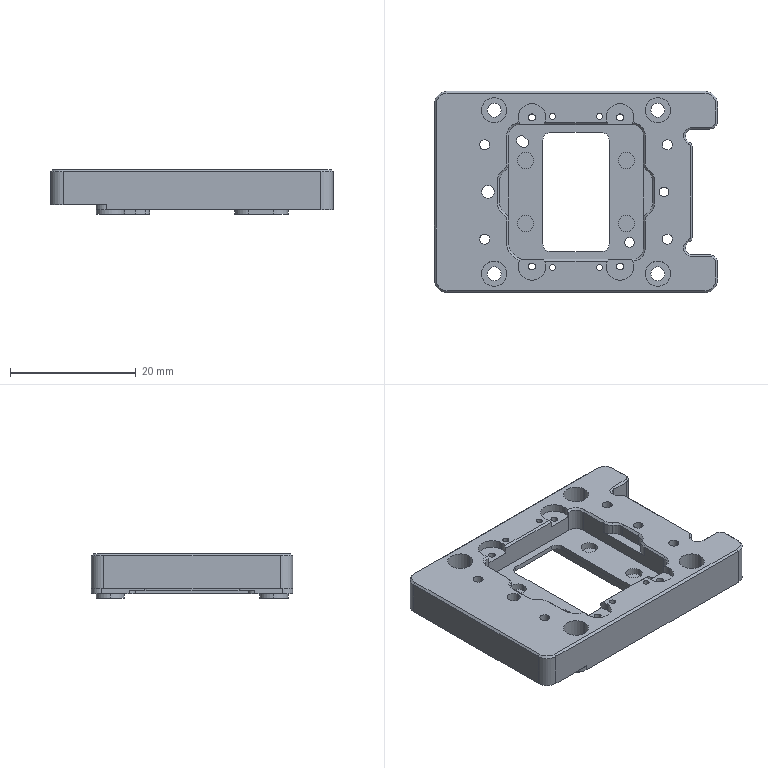NC program | NX | posted with a generic post | part box 45 x 32 x 7.05 mm
Lines 3844 to 5415 of 5787, first 1338 of 1564 lines:
(HOLE_MILLING_COPY , TOOL : D1.5)
N7602 T19 M6
N7604 G54
N7606 G17 G0 G90 X-8. Y5. S9500 M3
N7608 G43 Z30. H19
N7610 Z-3.35
N7612 G94 G3 X-7.725 Y4.725 R0.275 F950.
N7614 X-7.45 Y5. R0.275
N7616 X-7.45 Y5. Z-3.45 I-0.55 J0.
N7618 X-7.45 Y5. Z-3.55 I-0.55 J0.
N7620 X-7.45 Y5. Z-3.65 I-0.55 J0.
N7622 X-7.45 Y5. Z-3.75 I-0.55 J0.
N7624 X-7.45 Y5. Z-3.85 I-0.55 J0.
N7626 X-7.45 Y5. Z-3.95 I-0.55 J0.
N7628 X-7.45 Y5. Z-4.05 I-0.55 J0.
N7630 X-7.45 Y5. Z-4.15 I-0.55 J0.
N7632 X-7.45 Y5. Z-4.25 I-0.55 J0.
N7634 X-7.45 Y5. Z-4.35 I-0.55 J0.
N7636 X-7.45 Y5. Z-4.45 I-0.55 J0.
N7638 X-7.45 Y5. Z-4.55 I-0.55 J0.
N7640 X-7.45 Y5. Z-4.65 I-0.55 J0.
N7642 X-7.45 Y5. Z-4.75 I-0.55 J0.
N7644 X-7.45 Y5. Z-4.85 I-0.55 J0.
N7646 X-8.55 Y5. Z-4.9 I-0.55 J0.
N7648 X-8. Y4.45 R0.55
N7650 X-8.55 Y5. R-0.55
N7652 X-8.275 Y4.725 R0.275
N7654 X-8. Y5. R0.275
N7656 G0 Z30.
N7658 Y-5.
N7660 Z-3.35
N7662 G3 X-7.725 Y-5.275 R0.275
N7664 X-7.45 Y-5. R0.275
N7666 X-7.45 Y-5. Z-3.45 I-0.55 J0.
N7668 X-7.45 Y-5. Z-3.55 I-0.55 J0.
N7670 X-7.45 Y-5. Z-3.65 I-0.55 J0.
N7672 X-7.45 Y-5. Z-3.75 I-0.55 J0.
N7674 X-7.45 Y-5. Z-3.85 I-0.55 J0.
N7676 X-7.45 Y-5. Z-3.95 I-0.55 J0.
N7678 X-7.45 Y-5. Z-4.05 I-0.55 J0.
N7680 X-7.45 Y-5. Z-4.15 I-0.55 J0.
N7682 X-7.45 Y-5. Z-4.25 I-0.55 J0.
N7684 X-7.45 Y-5. Z-4.35 I-0.55 J0.
N7686 X-7.45 Y-5. Z-4.45 I-0.55 J0.
N7688 X-7.45 Y-5. Z-4.55 I-0.55 J0.
N7690 X-7.45 Y-5. Z-4.65 I-0.55 J0.
N7692 X-7.45 Y-5. Z-4.75 I-0.55 J0.
N7694 X-7.45 Y-5. Z-4.85 I-0.55 J0.
N7696 X-8.55 Y-5. Z-4.9 I-0.55 J0.
N7698 X-8. Y-5.55 R0.55
N7700 X-8.55 Y-5. R-0.55
N7702 X-8.275 Y-5.275 R0.275
N7704 X-8. Y-5. R0.275
N7706 G0 Z30.
N7708 X8.
N7710 Z-3.35
N7712 G3 X8.275 Y-5.275 R0.275
N7714 X8.55 Y-5. R0.275
N7716 X8.55 Y-5. Z-3.45 I-0.55 J0.
N7718 X8.55 Y-5. Z-3.55 I-0.55 J0.
N7720 X8.55 Y-5. Z-3.65 I-0.55 J0.
N7722 X8.55 Y-5. Z-3.75 I-0.55 J0.
N7724 X8.55 Y-5. Z-3.85 I-0.55 J0.
N7726 X8.55 Y-5. Z-3.95 I-0.55 J0.
N7728 X8.55 Y-5. Z-4.05 I-0.55 J0.
N7730 X8.55 Y-5. Z-4.15 I-0.55 J0.
N7732 X8.55 Y-5. Z-4.25 I-0.55 J0.
N7734 X8.55 Y-5. Z-4.35 I-0.55 J0.
N7736 X8.55 Y-5. Z-4.45 I-0.55 J0.
N7738 X8.55 Y-5. Z-4.55 I-0.55 J0.
N7740 X8.55 Y-5. Z-4.65 I-0.55 J0.
N7742 X8.55 Y-5. Z-4.75 I-0.55 J0.
N7744 X8.55 Y-5. Z-4.85 I-0.55 J0.
N7746 X7.45 Y-5. Z-4.9 I-0.55 J0.
N7748 X8. Y-5.55 R0.55
N7750 X7.45 Y-5. R-0.55
N7752 X7.725 Y-5.275 R0.275
N7754 X8. Y-5. R0.275
N7756 G0 Z30.
N7758 Y5.
N7760 Z-3.35
N7762 G3 X8.275 Y4.725 R0.275
N7764 X8.55 Y5. R0.275
N7766 X8.55 Y5. Z-3.45 I-0.55 J0.
N7768 X8.55 Y5. Z-3.55 I-0.55 J0.
N7770 X8.55 Y5. Z-3.65 I-0.55 J0.
N7772 X8.55 Y5. Z-3.75 I-0.55 J0.
N7774 X8.55 Y5. Z-3.85 I-0.55 J0.
N7776 X8.55 Y5. Z-3.95 I-0.55 J0.
N7778 X8.55 Y5. Z-4.05 I-0.55 J0.
N7780 X8.55 Y5. Z-4.15 I-0.55 J0.
N7782 X8.55 Y5. Z-4.25 I-0.55 J0.
N7784 X8.55 Y5. Z-4.35 I-0.55 J0.
N7786 X8.55 Y5. Z-4.45 I-0.55 J0.
N7788 X8.55 Y5. Z-4.55 I-0.55 J0.
N7790 X8.55 Y5. Z-4.65 I-0.55 J0.
N7792 X8.55 Y5. Z-4.75 I-0.55 J0.
N7794 X8.55 Y5. Z-4.85 I-0.55 J0.
N7796 X7.45 Y5. Z-4.9 I-0.55 J0.
N7798 X8. Y4.45 R0.55
N7800 X7.45 Y5. R-0.55
N7802 X7.725 Y4.725 R0.275
N7804 X8. Y5. R0.275
N7806 G0 Z30.
(CAVITY_MILL_COPY , TOOL : D1.5)
N7808 X-4.2 Y-7.103
N7810 Z-4.
N7812 G3 X-4.5 Y-7.817 R1.
N7814 G1 Y-8.25
N7816 G3 X-4. Y-8.75 R0.5
N7818 G1 X-3.567
N7820 G3 X-2.853 Y-8.45 R1.
N7822 G0 X-4.2 Y-7.103 Z-4.15
N7824 G3 X-4.5 Y-7.817 R1.
N7826 G1 Y-8.25
N7828 G3 X-4. Y-8.75 R0.5
N7830 G1 X-3.567
N7832 G3 X-2.853 Y-8.45 R1.
N7834 G0 X-4.2 Y-7.103 Z-4.3
N7836 G3 X-4.5 Y-7.817 R1.
N7838 G1 Y-8.25
N7840 G3 X-4. Y-8.75 R0.5
N7842 G1 X-3.567
N7844 G3 X-2.853 Y-8.45 R1.
N7846 G0 X-4.2 Y-7.103 Z-4.45
N7848 G3 X-4.5 Y-7.817 R1.
N7850 G1 Y-8.25
N7852 G3 X-4. Y-8.75 R0.5
N7854 G1 X-3.567
N7856 G3 X-2.853 Y-8.45 R1.
N7858 G0 X-4.2 Y-7.104 Z-4.6
N7860 G3 X-4.5 Y-7.818 R1.
N7862 G1 Y-8.25
N7864 G3 X-4. Y-8.75 R0.5
N7866 G1 X-3.568
N7868 G3 X-2.854 Y-8.45 R1.
N7870 G0 Z30.
N7872 X2.853
N7874 Z-4.
N7876 G3 X3.567 Y-8.75 R1.
N7878 G1 X4.
N7880 G3 X4.5 Y-8.25 R0.5
N7882 G1 Y-7.817
N7884 G3 X4.2 Y-7.103 R1.
N7886 G0 X2.853 Y-8.45 Z-4.15
N7888 G3 X3.567 Y-8.75 R1.
N7890 G1 X4.
N7892 G3 X4.5 Y-8.25 R0.5
N7894 G1 Y-7.817
N7896 G3 X4.2 Y-7.103 R1.
N7898 G0 X2.853 Y-8.45 Z-4.3
N7900 G3 X3.567 Y-8.75 R1.
N7902 G1 X4.
N7904 G3 X4.5 Y-8.25 R0.5
N7906 G1 Y-7.817
N7908 G3 X4.2 Y-7.103 R1.
N7910 G0 X2.853 Y-8.45 Z-4.45
N7912 G3 X3.567 Y-8.75 R1.
N7914 G1 X4.
N7916 G3 X4.5 Y-8.25 R0.5
N7918 G1 Y-7.817
N7920 G3 X4.2 Y-7.103 R1.
N7922 G0 X2.854 Y-8.45 Z-4.6
N7924 G3 X3.568 Y-8.75 R1.
N7926 G1 X4.
N7928 G3 X4.5 Y-8.25 R0.5
N7930 G1 Y-7.818
N7932 G3 X4.2 Y-7.104 R1.
N7934 G0 Z30.
N7936 Y7.103
N7938 Z-4.
N7940 G3 X4.5 Y7.817 R1.
N7942 G1 Y8.25
N7944 G3 X4. Y8.75 R0.5
N7946 G1 X3.567
N7948 G3 X2.853 Y8.45 R1.
N7950 G0 X4.2 Y7.103 Z-4.15
N7952 G3 X4.5 Y7.817 R1.
N7954 G1 Y8.25
N7956 G3 X4. Y8.75 R0.5
N7958 G1 X3.567
N7960 G3 X2.853 Y8.45 R1.
N7962 G0 X4.2 Y7.103 Z-4.3
N7964 G3 X4.5 Y7.817 R1.
N7966 G1 Y8.25
N7968 G3 X4. Y8.75 R0.5
N7970 G1 X3.567
N7972 G3 X2.853 Y8.45 R1.
N7974 G0 X4.2 Y7.103 Z-4.45
N7976 G3 X4.5 Y7.817 R1.
N7978 G1 Y8.25
N7980 G3 X4. Y8.75 R0.5
N7982 G1 X3.567
N7984 G3 X2.853 Y8.45 R1.
N7986 G0 X4.2 Y7.103 Z-4.6
N7988 G3 X4.5 Y7.817 R1.
N7990 G1 Y8.25
N7992 G3 X4. Y8.75 R0.5
N7994 G1 X3.567
N7996 G3 X2.853 Y8.45 R1.
N7998 G0 Z30.
N8000 X-2.853
N8002 Z-4.
N8004 G3 X-3.567 Y8.75 R1.
N8006 G1 X-4.
N8008 G3 X-4.5 Y8.25 R0.5
N8010 G1 Y7.817
N8012 G3 X-4.2 Y7.103 R1.
N8014 G0 X-2.853 Y8.45 Z-4.15
N8016 G3 X-3.567 Y8.75 R1.
N8018 G1 X-4.
N8020 G3 X-4.5 Y8.25 R0.5
N8022 G1 Y7.817
N8024 G3 X-4.2 Y7.103 R1.
N8026 G0 X-2.853 Y8.45 Z-4.3
N8028 G3 X-3.567 Y8.75 R1.
N8030 G1 X-4.
N8032 G3 X-4.5 Y8.25 R0.5
N8034 G1 Y7.817
N8036 G3 X-4.2 Y7.103 R1.
N8038 G0 X-2.853 Y8.45 Z-4.45
N8040 G3 X-3.567 Y8.75 R1.
N8042 G1 X-4.
N8044 G3 X-4.5 Y8.25 R0.5
N8046 G1 Y7.817
N8048 G3 X-4.2 Y7.103 R1.
N8050 G0 X-2.853 Y8.45 Z-4.6
N8052 G3 X-3.567 Y8.75 R1.
N8054 G1 X-4.
N8056 G3 X-4.5 Y8.25 R0.5
N8058 G1 Y7.817
N8060 G3 X-4.2 Y7.103 R1.
N8062 G0 Z30.
(CAVITY_MILL_COPY_COPY , TOOL : D1.5)
N8064 X20.107 Y9.111
N8066 Z-0.139
N8068 G3 X19.393 Y9.411 R1.
N8070 G1 X18.5
N8072 G3 X18.257 Y8.451 R0.511
N8074 G2 X18.811 Y7.952 R1.589
N8076 G3 X19.317 Y7.569 R1.
N8078 G0 X20.404 Y8.972 Z-0.278
N8080 G3 X19.69 Y9.272 R1.
N8082 G1 X18.5
N8084 G3 X18.323 Y8.573 R0.372
N8086 G2 X19.023 Y7.87 R1.728
N8088 G3 X19.492 Y7.431 R1.
N8090 G0 X20.447 Y8.95 Z-0.417
N8092 G3 X19.733 Y9.25 R1.
N8094 G1 X18.5
N8096 G3 X18.333 Y8.592 R0.35
N8098 G2 X19.055 Y7.856 R1.75
N8100 G3 X19.519 Y7.41 R1.
N8102 G0 X20.447 Y8.95 Z-0.556
N8104 G3 X19.733 Y9.25 R1.
N8106 G1 X18.5
N8108 G3 X18.333 Y8.592 R0.35
N8110 G2 X19.055 Y7.856 R1.75
N8112 G3 X19.519 Y7.41 R1.
N8114 G0 X20.447 Y8.95 Z-0.694
N8116 G3 X19.733 Y9.25 R1.
N8118 G1 X18.5
N8120 G3 X18.333 Y8.592 R0.35
N8122 G2 X19.055 Y7.856 R1.75
N8124 G3 X19.519 Y7.41 R1.
N8126 G0 X20.447 Y8.95 Z-0.833
N8128 G3 X19.733 Y9.25 R1.
N8130 G1 X18.5
N8132 G3 X18.333 Y8.592 R0.35
N8134 G2 X19.055 Y7.856 R1.75
N8136 G3 X19.519 Y7.41 R1.
N8138 G0 X20.447 Y8.95 Z-0.972
N8140 G3 X19.733 Y9.25 R1.
N8142 G1 X18.5
N8144 G3 X18.333 Y8.592 R0.35
N8146 G2 X19.055 Y7.856 R1.75
N8148 G3 X19.519 Y7.41 R1.
N8150 G0 X20.447 Y8.95 Z-1.111
N8152 G3 X19.733 Y9.25 R1.
N8154 G1 X18.5
N8156 G3 X18.333 Y8.592 R0.35
N8158 G2 X19.055 Y7.856 R1.75
N8160 G3 X19.519 Y7.41 R1.
N8162 G0 X20.447 Y8.95 Z-1.25
N8164 G3 X19.733 Y9.25 R1.
N8166 G1 X18.5
N8168 G3 X18.333 Y8.592 R0.35
N8170 G2 X19.055 Y7.856 R1.75
N8172 G3 X19.519 Y7.41 R1.
N8174 G0 X20.447 Y8.95 Z-1.4
N8176 G3 X19.733 Y9.25 R1.
N8178 G1 X18.5
N8180 G3 X18.333 Y8.592 R0.35
N8182 G2 X19.055 Y7.856 R1.75
N8184 G3 X19.519 Y7.41 R1.
N8186 G0 X20.447 Y8.95 Z-1.55
N8188 G3 X19.733 Y9.25 R1.
N8190 G1 X18.5
N8192 G3 X18.333 Y8.592 R0.35
N8194 G2 X19.055 Y7.856 R1.75
N8196 G3 X19.519 Y7.41 R1.
N8198 G0 X20.447 Y8.95 Z-1.7
N8200 G3 X19.733 Y9.25 R1.
N8202 G1 X18.5
N8204 G3 X18.333 Y8.592 R0.35
N8206 G2 X19.055 Y7.856 R1.75
N8208 G3 X19.519 Y7.41 R1.
N8210 G0 X20.447 Y8.95 Z-1.85
N8212 G3 X19.733 Y9.25 R1.
N8214 G1 X18.5
N8216 G3 X18.333 Y8.592 R0.35
N8218 G2 X19.055 Y7.856 R1.75
N8220 G3 X19.519 Y7.41 R1.
N8222 G0 X20.447 Y8.95 Z-2.
N8224 G3 X19.733 Y9.25 R1.
N8226 G1 X18.5
N8228 G3 X18.333 Y8.592 R0.35
N8230 G2 X19.055 Y7.856 R1.75
N8232 G3 X19.519 Y7.41 R1.
N8234 G0 X20.447 Y8.95 Z-2.143
N8236 G3 X19.733 Y9.25 R1.
N8238 G1 X18.5
N8240 G3 X18.333 Y8.592 R0.35
N8242 G2 X19.055 Y7.856 R1.75
N8244 G3 X19.519 Y7.41 R1.
N8246 G0 X20.447 Y8.95 Z-2.286
N8248 G3 X19.733 Y9.25 R1.
N8250 G1 X18.5
N8252 G3 X18.333 Y8.592 R0.35
N8254 G2 X19.055 Y7.856 R1.75
N8256 G3 X19.519 Y7.41 R1.
N8258 G0 X20.447 Y8.95 Z-2.429
N8260 G3 X19.733 Y9.25 R1.
N8262 G1 X18.5
N8264 G3 X18.333 Y8.592 R0.35
N8266 G2 X19.055 Y7.856 R1.75
N8268 G3 X19.519 Y7.41 R1.
N8270 G0 X20.447 Y8.95 Z-2.571
N8272 G3 X19.733 Y9.25 R1.
N8274 G1 X18.5
N8276 G3 X18.333 Y8.592 R0.35
N8278 G2 X19.055 Y7.856 R1.75
N8280 G3 X19.519 Y7.41 R1.
N8282 G0 X20.447 Y8.95 Z-2.714
N8284 G3 X19.733 Y9.25 R1.
N8286 G1 X18.5
N8288 G3 X18.333 Y8.592 R0.35
N8290 G2 X19.055 Y7.856 R1.75
N8292 G3 X19.519 Y7.41 R1.
N8294 G0 X20.447 Y8.95 Z-2.857
N8296 G3 X19.733 Y9.25 R1.
N8298 G1 X18.5
N8300 G3 X18.333 Y8.592 R0.35
N8302 G2 X19.055 Y7.856 R1.75
N8304 G3 X19.519 Y7.41 R1.
N8306 G0 X20.447 Y8.95 Z-3.
N8308 G3 X19.733 Y9.25 R1.
N8310 G1 X18.5
N8312 G3 X18.333 Y8.592 R0.35
N8314 G2 X19.055 Y7.856 R1.75
N8316 G3 X19.519 Y7.41 R1.
N8318 G0 X20.447 Y8.95 Z-3.142
N8320 G3 X19.733 Y9.25 R1.
N8322 G1 X18.5
N8324 G3 X18.333 Y8.592 R0.35
N8326 G2 X19.055 Y7.856 R1.75
N8328 G3 X19.519 Y7.41 R1.
N8330 G0 X20.447 Y8.95 Z-3.283
N8332 G3 X19.733 Y9.25 R1.
N8334 G1 X18.5
N8336 G3 X18.333 Y8.592 R0.35
N8338 G2 X19.055 Y7.856 R1.75
N8340 G3 X19.519 Y7.41 R1.
N8342 G0 X20.447 Y8.95 Z-3.425
N8344 G3 X19.733 Y9.25 R1.
N8346 G1 X18.5
N8348 G3 X18.333 Y8.592 R0.35
N8350 G2 X19.055 Y7.856 R1.75
N8352 G3 X19.519 Y7.41 R1.
N8354 G0 X20.447 Y8.95 Z-3.567
N8356 G3 X19.733 Y9.25 R1.
N8358 G1 X18.5
N8360 G3 X18.333 Y8.592 R0.35
N8362 G2 X19.055 Y7.856 R1.75
N8364 G3 X19.519 Y7.41 R1.
N8366 G0 X20.447 Y8.95 Z-3.708
N8368 G3 X19.733 Y9.25 R1.
N8370 G1 X18.5
N8372 G3 X18.333 Y8.592 R0.35
N8374 G2 X19.055 Y7.856 R1.75
N8376 G3 X19.519 Y7.41 R1.
N8378 G0 X20.447 Y8.95 Z-3.85
N8380 G3 X19.733 Y9.25 R1.
N8382 G1 X18.5
N8384 G3 X18.333 Y8.592 R0.35
N8386 G2 X19.055 Y7.856 R1.75
N8388 G3 X19.519 Y7.41 R1.
N8390 G0 X20.447 Y8.95 Z-4.
N8392 G3 X19.733 Y9.25 R1.
N8394 G1 X18.5
N8396 G3 X18.333 Y8.592 R0.35
N8398 G2 X19.055 Y7.856 R1.75
N8400 G3 X19.519 Y7.41 R1.
N8402 G0 X20.447 Y8.95 Z-4.15
N8404 G3 X19.733 Y9.25 R1.
N8406 G1 X18.5
N8408 G3 X18.333 Y8.592 R0.35
N8410 G2 X19.055 Y7.856 R1.75
N8412 G3 X19.519 Y7.41 R1.
N8414 G0 X20.447 Y8.95 Z-4.3
N8416 G3 X19.733 Y9.25 R1.
N8418 G1 X18.5
N8420 G3 X18.333 Y8.592 R0.35
N8422 G2 X19.055 Y7.856 R1.75
N8424 G3 X19.519 Y7.41 R1.
N8426 G0 X20.447 Y8.95 Z-4.45
N8428 G3 X19.733 Y9.25 R1.
N8430 G1 X18.5
N8432 G3 X18.333 Y8.592 R0.35
N8434 G2 X19.055 Y7.856 R1.75
N8436 G3 X19.519 Y7.41 R1.
N8438 G0 X20.447 Y8.95 Z-4.6
N8440 G3 X19.733 Y9.25 R1.
N8442 G1 X18.5
N8444 G3 X18.333 Y8.592 R0.35
N8446 G2 X19.055 Y7.856 R1.75
N8448 G3 X19.519 Y7.41 R1.
N8450 G0 X20.447 Y8.95 Z-4.75
N8452 G3 X19.733 Y9.25 R1.
N8454 G1 X18.5
N8456 G3 X18.333 Y8.592 R0.35
N8458 G2 X19.055 Y7.856 R1.75
N8460 G3 X19.519 Y7.41 R1.
N8462 G0 X20.447 Y8.95 Z-4.9
N8464 G3 X19.733 Y9.25 R1.
N8466 G1 X18.5
N8468 G3 X18.333 Y8.592 R0.35
N8470 G2 X19.055 Y7.856 R1.75
N8472 G3 X19.519 Y7.41 R1.
N8474 G0 X20.447 Y8.95 Z-5.043
N8476 G3 X19.733 Y9.25 R1.
N8478 G1 X18.5
N8480 G3 X18.333 Y8.592 R0.35
N8482 G2 X19.055 Y7.856 R1.75
N8484 G3 X19.519 Y7.41 R1.
N8486 G0 X20.447 Y8.95 Z-5.187
N8488 G3 X19.733 Y9.25 R1.
N8490 G1 X18.5
N8492 G3 X18.333 Y8.592 R0.35
N8494 G2 X19.055 Y7.856 R1.75
N8496 G3 X19.519 Y7.41 R1.
N8498 G0 X20.447 Y8.95 Z-5.33
N8500 G3 X19.733 Y9.25 R1.
N8502 G1 X18.5
N8504 G3 X18.333 Y8.592 R0.35
N8506 G2 X19.055 Y7.856 R1.75
N8508 G3 X19.519 Y7.41 R1.
N8510 G0 X20.447 Y8.95 Z-5.473
N8512 G3 X19.733 Y9.25 R1.
N8514 G1 X18.5
N8516 G3 X18.333 Y8.592 R0.35
N8518 G2 X19.055 Y7.856 R1.75
N8520 G3 X19.519 Y7.41 R1.
N8522 G0 X20.447 Y8.95 Z-5.617
N8524 G3 X19.733 Y9.25 R1.
N8526 G1 X18.5
N8528 G3 X18.333 Y8.592 R0.35
N8530 G2 X19.055 Y7.856 R1.75
N8532 G3 X19.519 Y7.41 R1.
N8534 G0 X20.447 Y8.95 Z-5.76
N8536 G3 X19.733 Y9.25 R1.
N8538 G1 X18.5
N8540 G3 X18.333 Y8.592 R0.35
N8542 G2 X19.055 Y7.856 R1.75
N8544 G3 X19.519 Y7.41 R1.
N8546 G0 X20.447 Y8.95 Z-5.903
N8548 G3 X19.733 Y9.25 R1.
N8550 G1 X18.5
N8552 G3 X18.333 Y8.592 R0.35
N8554 G2 X19.055 Y7.856 R1.75
N8556 G3 X19.519 Y7.41 R1.
N8558 G0 X20.447 Y8.95 Z-6.047
N8560 G3 X19.733 Y9.25 R1.
N8562 G1 X18.5
N8564 G3 X18.333 Y8.592 R0.35
N8566 G2 X19.055 Y7.856 R1.75
N8568 G3 X19.519 Y7.41 R1.
N8570 G0 X20.447 Y8.95 Z-6.19
N8572 G3 X19.733 Y9.25 R1.
N8574 G1 X18.5
N8576 G3 X18.333 Y8.592 R0.35
N8578 G2 X19.055 Y7.856 R1.75
N8580 G3 X19.519 Y7.41 R1.
N8582 G0 X20.447 Y8.95 Z-6.333
N8584 G3 X19.733 Y9.25 R1.
N8586 G1 X18.5
N8588 G3 X18.333 Y8.592 R0.35
N8590 G2 X19.055 Y7.856 R1.75
N8592 G3 X19.519 Y7.41 R1.
N8594 G0 X20.469 Y8.95 Z-6.477
N8596 G3 X19.755 Y9.25 R1.
N8598 G1 X18.5
N8600 G3 X18.333 Y8.592 R0.35
N8602 G2 X19.074 Y7.818 R1.75
N8604 G3 X19.527 Y7.36 R1.
N8606 G0 X20.469 Y8.95 Z-6.62
N8608 G3 X19.755 Y9.25 R1.
N8610 G1 X18.5
N8612 G3 X18.333 Y8.592 R0.35
N8614 G2 X19.074 Y7.818 R1.75
N8616 G3 X19.527 Y7.36 R1.
N8618 G0 X20.469 Y8.95 Z-6.763
N8620 G3 X19.755 Y9.25 R1.
N8622 G1 X18.5
N8624 G3 X18.333 Y8.592 R0.35
N8626 G2 X19.074 Y7.818 R1.75
N8628 G3 X19.527 Y7.36 R1.
N8630 G0 X20.469 Y8.95 Z-6.907
N8632 G3 X19.755 Y9.25 R1.
N8634 G1 X18.5
N8636 G3 X18.333 Y8.592 R0.35
N8638 G2 X19.074 Y7.818 R1.75
N8640 G3 X19.527 Y7.36 R1.
N8642 G0 X20.469 Y8.95 Z-7.05
N8644 G3 X19.755 Y9.25 R1.
N8646 G1 X18.5
N8648 G3 X18.333 Y8.592 R0.35
N8650 G2 X19.074 Y7.818 R1.75
N8652 G3 X19.527 Y7.36 R1.
N8654 G0 Z30.
N8656 X19.317 Y-7.569
N8658 Z-0.139
N8660 G3 X18.811 Y-7.952 R1.
N8662 G2 X18.257 Y-8.451 R1.589
N8664 G3 X18.5 Y-9.411 R0.511
N8666 G1 X19.393
N8668 G3 X20.107 Y-9.111 R1.
N8670 G0 X19.492 Y-7.431 Z-0.278
N8672 G3 X19.023 Y-7.87 R1.
N8674 G2 X18.323 Y-8.573 R1.728
N8676 G3 X18.5 Y-9.272 R0.372
N8678 G1 X19.69
N8680 G3 X20.404 Y-8.972 R1.
N8682 G0 X19.519 Y-7.41 Z-0.417
N8684 G3 X19.055 Y-7.856 R1.
N8686 G2 X18.333 Y-8.592 R1.75
N8688 G3 X18.5 Y-9.25 R0.35
N8690 G1 X19.733
N8692 G3 X20.447 Y-8.95 R1.
N8694 G0 X19.519 Y-7.41 Z-0.556
N8696 G3 X19.055 Y-7.856 R1.
N8698 G2 X18.333 Y-8.592 R1.75
N8700 G3 X18.5 Y-9.25 R0.35
N8702 G1 X19.733
N8704 G3 X20.447 Y-8.95 R1.
N8706 G0 X19.519 Y-7.41 Z-0.694
N8708 G3 X19.055 Y-7.856 R1.
N8710 G2 X18.333 Y-8.592 R1.75
N8712 G3 X18.5 Y-9.25 R0.35
N8714 G1 X19.733
N8716 G3 X20.447 Y-8.95 R1.
N8718 G0 X19.519 Y-7.41 Z-0.833
N8720 G3 X19.055 Y-7.856 R1.
N8722 G2 X18.333 Y-8.592 R1.75
N8724 G3 X18.5 Y-9.25 R0.35
N8726 G1 X19.733
N8728 G3 X20.447 Y-8.95 R1.
N8730 G0 X19.519 Y-7.41 Z-0.972
N8732 G3 X19.055 Y-7.856 R1.
N8734 G2 X18.333 Y-8.592 R1.75
N8736 G3 X18.5 Y-9.25 R0.35
N8738 G1 X19.733
N8740 G3 X20.447 Y-8.95 R1.
N8742 G0 X19.519 Y-7.41 Z-1.111
N8744 G3 X19.055 Y-7.856 R1.
N8746 G2 X18.333 Y-8.592 R1.75
N8748 G3 X18.5 Y-9.25 R0.35
N8750 G1 X19.733
N8752 G3 X20.447 Y-8.95 R1.
N8754 G0 X19.519 Y-7.41 Z-1.25
N8756 G3 X19.055 Y-7.856 R1.
N8758 G2 X18.333 Y-8.592 R1.75
N8760 G3 X18.5 Y-9.25 R0.35
N8762 G1 X19.733
N8764 G3 X20.447 Y-8.95 R1.
N8766 G0 X19.519 Y-7.41 Z-1.4
N8768 G3 X19.055 Y-7.856 R1.
N8770 G2 X18.333 Y-8.592 R1.75
N8772 G3 X18.5 Y-9.25 R0.35
N8774 G1 X19.733
N8776 G3 X20.447 Y-8.95 R1.
N8778 G0 X19.519 Y-7.41 Z-1.55
N8780 G3 X19.055 Y-7.856 R1.
N8782 G2 X18.333 Y-8.592 R1.75
N8784 G3 X18.5 Y-9.25 R0.35
N8786 G1 X19.733
N8788 G3 X20.447 Y-8.95 R1.
N8790 G0 X19.519 Y-7.41 Z-1.7
N8792 G3 X19.055 Y-7.856 R1.
N8794 G2 X18.333 Y-8.592 R1.75
N8796 G3 X18.5 Y-9.25 R0.35
N8798 G1 X19.733
N8800 G3 X20.447 Y-8.95 R1.
N8802 G0 X19.519 Y-7.41 Z-1.85
N8804 G3 X19.055 Y-7.856 R1.
N8806 G2 X18.333 Y-8.592 R1.75
N8808 G3 X18.5 Y-9.25 R0.35
N8810 G1 X19.733
N8812 G3 X20.447 Y-8.95 R1.
N8814 G0 X19.519 Y-7.41 Z-2.
N8816 G3 X19.055 Y-7.856 R1.
N8818 G2 X18.333 Y-8.592 R1.75
N8820 G3 X18.5 Y-9.25 R0.35
N8822 G1 X19.733
N8824 G3 X20.447 Y-8.95 R1.
N8826 G0 X19.519 Y-7.41 Z-2.143
N8828 G3 X19.055 Y-7.856 R1.
N8830 G2 X18.333 Y-8.592 R1.75
N8832 G3 X18.5 Y-9.25 R0.35
N8834 G1 X19.733
N8836 G3 X20.447 Y-8.95 R1.
N8838 G0 X19.519 Y-7.41 Z-2.286
N8840 G3 X19.055 Y-7.856 R1.
N8842 G2 X18.333 Y-8.592 R1.75
N8844 G3 X18.5 Y-9.25 R0.35
N8846 G1 X19.733
N8848 G3 X20.447 Y-8.95 R1.
N8850 G0 X19.519 Y-7.41 Z-2.429
N8852 G3 X19.055 Y-7.856 R1.
N8854 G2 X18.333 Y-8.592 R1.75
N8856 G3 X18.5 Y-9.25 R0.35
N8858 G1 X19.733
N8860 G3 X20.447 Y-8.95 R1.
N8862 G0 X19.519 Y-7.41 Z-2.571
N8864 G3 X19.055 Y-7.856 R1.
N8866 G2 X18.333 Y-8.592 R1.75
N8868 G3 X18.5 Y-9.25 R0.35
N8870 G1 X19.733
N8872 G3 X20.447 Y-8.95 R1.
N8874 G0 X19.519 Y-7.41 Z-2.714
N8876 G3 X19.055 Y-7.856 R1.
N8878 G2 X18.333 Y-8.592 R1.75
N8880 G3 X18.5 Y-9.25 R0.35
N8882 G1 X19.733
N8884 G3 X20.447 Y-8.95 R1.
N8886 G0 X19.519 Y-7.41 Z-2.857
N8888 G3 X19.055 Y-7.856 R1.
N8890 G2 X18.333 Y-8.592 R1.75
N8892 G3 X18.5 Y-9.25 R0.35
N8894 G1 X19.733
N8896 G3 X20.447 Y-8.95 R1.
N8898 G0 X19.519 Y-7.41 Z-3.
N8900 G3 X19.055 Y-7.856 R1.
N8902 G2 X18.333 Y-8.592 R1.75
N8904 G3 X18.5 Y-9.25 R0.35
N8906 G1 X19.733
N8908 G3 X20.447 Y-8.95 R1.
N8910 G0 X19.519 Y-7.41 Z-3.142
N8912 G3 X19.055 Y-7.856 R1.
N8914 G2 X18.333 Y-8.592 R1.75
N8916 G3 X18.5 Y-9.25 R0.35
N8918 G1 X19.733
N8920 G3 X20.447 Y-8.95 R1.
N8922 G0 X19.519 Y-7.41 Z-3.283
N8924 G3 X19.055 Y-7.856 R1.
N8926 G2 X18.333 Y-8.592 R1.75
N8928 G3 X18.5 Y-9.25 R0.35
N8930 G1 X19.733
N8932 G3 X20.447 Y-8.95 R1.
N8934 G0 X19.519 Y-7.41 Z-3.425
N8936 G3 X19.055 Y-7.856 R1.
N8938 G2 X18.333 Y-8.592 R1.75
N8940 G3 X18.5 Y-9.25 R0.35
N8942 G1 X19.733
N8944 G3 X20.447 Y-8.95 R1.
N8946 G0 X19.519 Y-7.41 Z-3.567
N8948 G3 X19.055 Y-7.856 R1.
N8950 G2 X18.333 Y-8.592 R1.75
N8952 G3 X18.5 Y-9.25 R0.35
N8954 G1 X19.733
N8956 G3 X20.447 Y-8.95 R1.
N8958 G0 X19.519 Y-7.41 Z-3.708
N8960 G3 X19.055 Y-7.856 R1.
N8962 G2 X18.333 Y-8.592 R1.75
N8964 G3 X18.5 Y-9.25 R0.35
N8966 G1 X19.733
N8968 G3 X20.447 Y-8.95 R1.
N8970 G0 X19.519 Y-7.41 Z-3.85
N8972 G3 X19.055 Y-7.856 R1.
N8974 G2 X18.333 Y-8.592 R1.75
N8976 G3 X18.5 Y-9.25 R0.35
N8978 G1 X19.733
N8980 G3 X20.447 Y-8.95 R1.
N8982 G0 X19.519 Y-7.41 Z-4.
N8984 G3 X19.055 Y-7.856 R1.
N8986 G2 X18.333 Y-8.592 R1.75
N8988 G3 X18.5 Y-9.25 R0.35
N8990 G1 X19.733
N8992 G3 X20.447 Y-8.95 R1.
N8994 G0 X19.519 Y-7.41 Z-4.15
N8996 G3 X19.055 Y-7.856 R1.
N8998 G2 X18.333 Y-8.592 R1.75
N9000 G3 X18.5 Y-9.25 R0.35
N9002 G1 X19.733
N9004 G3 X20.447 Y-8.95 R1.
N9006 G0 X19.519 Y-7.41 Z-4.3
N9008 G3 X19.055 Y-7.856 R1.
N9010 G2 X18.333 Y-8.592 R1.75
N9012 G3 X18.5 Y-9.25 R0.35
N9014 G1 X19.733
N9016 G3 X20.447 Y-8.95 R1.
N9018 G0 X19.519 Y-7.41 Z-4.45
N9020 G3 X19.055 Y-7.856 R1.
N9022 G2 X18.333 Y-8.592 R1.75
N9024 G3 X18.5 Y-9.25 R0.35
N9026 G1 X19.733
N9028 G3 X20.447 Y-8.95 R1.
N9030 G0 X19.519 Y-7.41 Z-4.6
N9032 G3 X19.055 Y-7.856 R1.
N9034 G2 X18.333 Y-8.592 R1.75
N9036 G3 X18.5 Y-9.25 R0.35
N9038 G1 X19.733
N9040 G3 X20.447 Y-8.95 R1.
N9042 G0 X19.519 Y-7.41 Z-4.75
N9044 G3 X19.055 Y-7.856 R1.
N9046 G2 X18.333 Y-8.592 R1.75
N9048 G3 X18.5 Y-9.25 R0.35
N9050 G1 X19.733
N9052 G3 X20.447 Y-8.95 R1.
N9054 G0 X19.519 Y-7.41 Z-4.9
N9056 G3 X19.055 Y-7.856 R1.
N9058 G2 X18.333 Y-8.592 R1.75
N9060 G3 X18.5 Y-9.25 R0.35
N9062 G1 X19.733
N9064 G3 X20.447 Y-8.95 R1.
N9066 G0 X19.519 Y-7.41 Z-5.043
N9068 G3 X19.055 Y-7.856 R1.
N9070 G2 X18.333 Y-8.592 R1.75
N9072 G3 X18.5 Y-9.25 R0.35
N9074 G1 X19.733
N9076 G3 X20.447 Y-8.95 R1.
N9078 G0 X19.519 Y-7.41 Z-5.187
N9080 G3 X19.055 Y-7.856 R1.
N9082 G2 X18.333 Y-8.592 R1.75
N9084 G3 X18.5 Y-9.25 R0.35
N9086 G1 X19.733
N9088 G3 X20.447 Y-8.95 R1.
N9090 G0 X19.519 Y-7.41 Z-5.33
N9092 G3 X19.055 Y-7.856 R1.
N9094 G2 X18.333 Y-8.592 R1.75
N9096 G3 X18.5 Y-9.25 R0.35
N9098 G1 X19.733
N9100 G3 X20.447 Y-8.95 R1.
N9102 G0 X19.519 Y-7.41 Z-5.473
N9104 G3 X19.055 Y-7.856 R1.
N9106 G2 X18.333 Y-8.592 R1.75
N9108 G3 X18.5 Y-9.25 R0.35
N9110 G1 X19.733
N9112 G3 X20.447 Y-8.95 R1.
N9114 G0 X19.519 Y-7.41 Z-5.617
N9116 G3 X19.055 Y-7.856 R1.
N9118 G2 X18.333 Y-8.592 R1.75
N9120 G3 X18.5 Y-9.25 R0.35
N9122 G1 X19.733
N9124 G3 X20.447 Y-8.95 R1.
N9126 G0 X19.519 Y-7.41 Z-5.76
N9128 G3 X19.055 Y-7.856 R1.
N9130 G2 X18.333 Y-8.592 R1.75
N9132 G3 X18.5 Y-9.25 R0.35
N9134 G1 X19.733
N9136 G3 X20.447 Y-8.95 R1.
N9138 G0 X19.519 Y-7.41 Z-5.903
N9140 G3 X19.055 Y-7.856 R1.
N9142 G2 X18.333 Y-8.592 R1.75
N9144 G3 X18.5 Y-9.25 R0.35
N9146 G1 X19.733
N9148 G3 X20.447 Y-8.95 R1.
N9150 G0 X19.519 Y-7.41 Z-6.047
N9152 G3 X19.055 Y-7.856 R1.
N9154 G2 X18.333 Y-8.592 R1.75
N9156 G3 X18.5 Y-9.25 R0.35
N9158 G1 X19.733
N9160 G3 X20.447 Y-8.95 R1.
N9162 G0 X19.519 Y-7.41 Z-6.19
N9164 G3 X19.055 Y-7.856 R1.
N9166 G2 X18.333 Y-8.592 R1.75
N9168 G3 X18.5 Y-9.25 R0.35
N9170 G1 X19.733
N9172 G3 X20.447 Y-8.95 R1.
N9174 G0 X19.519 Y-7.41 Z-6.333
N9176 G3 X19.055 Y-7.856 R1.
N9178 G2 X18.333 Y-8.592 R1.75
N9180 G3 X18.5 Y-9.25 R0.35
N9182 G1 X19.733
N9184 G3 X20.447 Y-8.95 R1.
N9186 G0 X19.527 Y-7.36 Z-6.477
N9188 G3 X19.074 Y-7.818 R1.
N9190 G2 X18.333 Y-8.592 R1.75
N9192 G3 X18.5 Y-9.25 R0.35
N9194 G1 X19.755
N9196 G3 X20.469 Y-8.95 R1.
N9198 G0 X19.527 Y-7.36 Z-6.62
N9200 G3 X19.074 Y-7.818 R1.
N9202 G2 X18.333 Y-8.592 R1.75
N9204 G3 X18.5 Y-9.25 R0.35
N9206 G1 X19.755
N9208 G3 X20.469 Y-8.95 R1.
N9210 G0 X19.527 Y-7.36 Z-6.763
N9212 G3 X19.074 Y-7.818 R1.
N9214 G2 X18.333 Y-8.592 R1.75
N9216 G3 X18.5 Y-9.25 R0.35
N9218 G1 X19.755
N9220 G3 X20.469 Y-8.95 R1.
N9222 G0 X19.527 Y-7.36 Z-6.907
N9224 G3 X19.074 Y-7.818 R1.
N9226 G2 X18.333 Y-8.592 R1.75
N9228 G3 X18.5 Y-9.25 R0.35
N9230 G1 X19.755
N9232 G3 X20.469 Y-8.95 R1.
N9234 G0 X19.527 Y-7.36 Z-7.05
N9236 G3 X19.074 Y-7.818 R1.
N9238 G2 X18.333 Y-8.592 R1.75
N9240 G3 X18.5 Y-9.25 R0.35
N9242 G1 X19.755
N9244 G3 X20.469 Y-8.95 R1.
N9246 G0 Z30.
N9248 M5
(ZLEVEL_PROFILE_1 , TOOL : D1)
N9250 T21 M6
N9252 G54
N9254 G17 G0 G90 X-8.667 Y7.848 S9500 M3
N9256 G43 Z30. H21
N9258 Z-3.35
N9260 G94 G1 X-8.423 Y7.618 Z-3.368 F850.
N9262 X-8.289 Y7.595 Z-3.375
N9264 X-8.165 Y7.65 Z-3.382
N9266 X-8.095 Y7.759 Z-3.389
N9268 X-8.091 Y7.889 Z-3.395
N9270 X-8.114 Y7.946 Z-3.399
N9272 X-8.579 Y8.383 Z-3.432
N9274 X-8.713 Y8.404 Z-3.439
N9276 X-8.844 Y8.341 Z-3.447
N9278 X-8.913 Y8.213 Z-3.454
N9280 X-8.898 Y8.078 Z-3.462
N9282 X-8.886 Y8.054 Z-3.463
N9284 X-8.423 Y7.618 Z-3.496
N9286 X-8.289 Y7.595 Z-3.503
N9288 X-8.165 Y7.65 Z-3.51
N9290 X-8.095 Y7.759 Z-3.517
N9292 X-8.091 Y7.889 Z-3.524
N9294 X-8.114 Y7.946 Z-3.527
N9296 X-8.579 Y8.383 Z-3.561
N9298 X-8.713 Y8.404 Z-3.568
N9300 X-8.844 Y8.341 Z-3.575
N9302 X-8.913 Y8.213 Z-3.583
N9304 X-8.898 Y8.078 Z-3.59
N9306 X-8.886 Y8.054 Z-3.592
N9308 X-8.423 Y7.618 Z-3.625
N9310 X-8.289 Y7.595 Z-3.632
N9312 X-8.165 Y7.65 Z-3.639
N9314 X-8.095 Y7.759 Z-3.646
N9316 X-8.091 Y7.889 Z-3.653
N9318 X-8.114 Y7.946 Z-3.656
N9320 X-8.579 Y8.383 Z-3.689
N9322 X-8.713 Y8.404 Z-3.697
N9324 X-8.844 Y8.341 Z-3.704
N9326 X-8.913 Y8.213 Z-3.712
N9328 X-8.898 Y8.078 Z-3.719
N9330 X-8.886 Y8.054 Z-3.72
N9332 X-8.423 Y7.618 Z-3.754
N9334 X-8.289 Y7.595 Z-3.761
N9336 X-8.165 Y7.65 Z-3.768
N9338 X-8.095 Y7.759 Z-3.775
N9340 X-8.091 Y7.889 Z-3.781
N9342 X-8.114 Y7.946 Z-3.785
N9344 X-8.579 Y8.383 Z-3.818
N9346 X-8.713 Y8.404 Z-3.825
N9348 X-8.844 Y8.341 Z-3.833
N9350 X-8.913 Y8.213 Z-3.84
N9352 X-8.898 Y8.078 Z-3.848
N9354 X-8.886 Y8.054 Z-3.849
N9356 X-8.423 Y7.618 Z-3.882
N9358 X-8.289 Y7.595 Z-3.889
N9360 X-8.165 Y7.65 Z-3.897
N9362 X-8.095 Y7.759 Z-3.903
N9364 X-8.091 Y7.889 Z-3.91
N9366 X-8.114 Y7.946 Z-3.913
N9368 X-8.346 Y8.164 Z-3.93
N9370 X-8.528 Y8.335
N9372 G3 X-8.846 Y8.326 R0.225
N9374 X-8.836 Y8.007 R0.225
N9376 G1 X-8.472 Y7.665
N9378 G3 X-8.154 Y7.674 R0.225
N9380 X-8.164 Y7.993 R0.225
N9382 G1 X-8.346 Y8.164
N9384 X-8.447 Y8.259 Z-3.936
N9386 X-8.535 Y8.333 Z-3.941
N9388 X-8.555 Y8.347 Z-3.942
N9390 X-8.61 Y8.376 Z-3.945
N9392 X-8.652 Y8.389 Z-3.947
N9394 X-8.68 Y8.388 Z-3.948
N9396 X-8.742 Y8.38 Z-3.951
N9398 X-8.783 Y8.366 Z-3.953
N9400 X-8.806 Y8.349 Z-3.955
N9402 X-8.87 Y8.281 Z-3.959
N9404 X-8.887 Y8.244 Z-3.961
N9406 X-8.898 Y8.167 Z-3.964
N9408 X-8.892 Y8.112 Z-3.967
N9410 X-8.874 Y8.065 Z-3.969
N9412 X-8.821 Y7.997 Z-3.973
N9414 X-8.773 Y7.948 Z-3.976
N9416 X-8.519 Y7.709 Z-3.992
N9418 X-8.433 Y7.642 Z-3.996
N9420 X-8.408 Y7.629 Z-3.998
N9422 X-8.328 Y7.611 Z-4.001
N9424 X-8.275 Y7.614 Z-4.004
N9426 X-8.242 Y7.624 Z-4.005
N9428 X-8.208 Y7.632 Z-4.007
N9430 X-8.18 Y7.651 Z-4.008
N9432 X-8.154 Y7.674 Z-4.01
N9434 G3 X-8.164 Y7.993 R0.225
N9436 G1 X-8.346 Y8.164
N9438 X-8.447 Y8.259 Z-4.016
N9440 X-8.535 Y8.333 Z-4.021
N9442 X-8.555 Y8.347 Z-4.022
N9444 X-8.61 Y8.376 Z-4.025
N9446 X-8.652 Y8.389 Z-4.027
N9448 X-8.68 Y8.388 Z-4.028
N9450 X-8.742 Y8.38 Z-4.031
N9452 X-8.783 Y8.366 Z-4.033
N9454 X-8.806 Y8.349 Z-4.035
N9456 X-8.87 Y8.281 Z-4.039
N9458 X-8.887 Y8.244 Z-4.041
N9460 X-8.898 Y8.167 Z-4.044
N9462 X-8.892 Y8.112 Z-4.047
N9464 X-8.874 Y8.065 Z-4.049
N9466 X-8.821 Y7.997 Z-4.053
N9468 X-8.773 Y7.948 Z-4.056
N9470 X-8.519 Y7.709 Z-4.072
N9472 X-8.433 Y7.642 Z-4.076
N9474 X-8.408 Y7.629 Z-4.078
N9476 X-8.328 Y7.611 Z-4.081
N9478 X-8.275 Y7.614 Z-4.084
N9480 X-8.242 Y7.624 Z-4.085
N9482 X-8.208 Y7.632 Z-4.087
N9484 X-8.18 Y7.651 Z-4.088
N9486 X-8.154 Y7.674 Z-4.09
N9488 G3 X-8.164 Y7.993 R0.225
N9490 G1 X-8.346 Y8.164
N9492 X-8.447 Y8.259 Z-4.096
N9494 X-8.535 Y8.333 Z-4.101
N9496 X-8.555 Y8.347 Z-4.102
N9498 X-8.61 Y8.376 Z-4.105
N9500 X-8.652 Y8.389 Z-4.107
N9502 X-8.68 Y8.388 Z-4.108
N9504 X-8.742 Y8.38 Z-4.111
N9506 X-8.783 Y8.366 Z-4.113
N9508 X-8.806 Y8.349 Z-4.115
N9510 X-8.87 Y8.281 Z-4.119
N9512 X-8.887 Y8.244 Z-4.121
N9514 X-8.898 Y8.167 Z-4.124
N9516 X-8.891 Y8.112 Z-4.127
N9518 X-8.874 Y8.065 Z-4.129
N9520 X-8.821 Y7.997 Z-4.133
N9522 X-8.773 Y7.948 Z-4.136
N9524 X-8.519 Y7.709 Z-4.152
N9526 X-8.433 Y7.642 Z-4.156
N9528 X-8.408 Y7.629 Z-4.158
N9530 X-8.328 Y7.611 Z-4.161
N9532 X-8.275 Y7.614 Z-4.164
N9534 X-8.242 Y7.624 Z-4.165
N9536 X-8.208 Y7.632 Z-4.167
N9538 X-8.18 Y7.651 Z-4.168
N9540 X-8.154 Y7.674 Z-4.17
N9542 G3 X-8.164 Y7.993 R0.225
N9544 G1 X-8.346 Y8.164
N9546 X-8.447 Y8.259 Z-4.176
N9548 X-8.535 Y8.333 Z-4.181
N9550 X-8.555 Y8.347 Z-4.182
N9552 X-8.61 Y8.376 Z-4.185
N9554 X-8.652 Y8.389 Z-4.187
N9556 X-8.68 Y8.388 Z-4.188
N9558 X-8.742 Y8.38 Z-4.191
N9560 X-8.783 Y8.366 Z-4.193
N9562 X-8.806 Y8.349 Z-4.195
N9564 X-8.87 Y8.281 Z-4.199
N9566 X-8.887 Y8.244 Z-4.201
N9568 X-8.898 Y8.167 Z-4.204
N9570 X-8.891 Y8.112 Z-4.207
N9572 X-8.874 Y8.065 Z-4.209
N9574 X-8.821 Y7.997 Z-4.213
N9576 X-8.773 Y7.948 Z-4.216
N9578 X-8.519 Y7.709 Z-4.232
N9580 X-8.433 Y7.642 Z-4.236
N9582 X-8.408 Y7.629 Z-4.238
N9584 X-8.328 Y7.611 Z-4.241
N9586 X-8.275 Y7.614 Z-4.244
N9588 X-8.242 Y7.624 Z-4.245
N9590 X-8.208 Y7.632 Z-4.247
N9592 X-8.18 Y7.651 Z-4.248
N9594 X-8.154 Y7.674 Z-4.25
N9596 G3 X-8.164 Y7.993 R0.225
N9598 G1 X-8.346 Y8.164
N9600 X-8.447 Y8.259 Z-4.256
N9602 X-8.535 Y8.333 Z-4.261
N9604 X-8.555 Y8.347 Z-4.262
N9606 X-8.61 Y8.376 Z-4.265
N9608 X-8.652 Y8.389 Z-4.267
N9610 X-8.68 Y8.388 Z-4.268
N9612 X-8.742 Y8.38 Z-4.271
N9614 X-8.783 Y8.366 Z-4.273
N9616 X-8.806 Y8.349 Z-4.275
N9618 X-8.87 Y8.281 Z-4.279
N9620 X-8.887 Y8.244 Z-4.281
N9622 X-8.898 Y8.167 Z-4.284
N9624 X-8.891 Y8.112 Z-4.287
N9626 X-8.874 Y8.065 Z-4.289
N9628 X-8.821 Y7.997 Z-4.293
N9630 X-8.773 Y7.948 Z-4.296
N9632 X-8.519 Y7.709 Z-4.312
N9634 X-8.433 Y7.642 Z-4.316
N9636 X-8.408 Y7.629 Z-4.318
N9638 X-8.328 Y7.611 Z-4.321
N9640 X-8.275 Y7.614 Z-4.324
N9642 X-8.242 Y7.624 Z-4.325
N9644 X-8.208 Y7.632 Z-4.327
N9646 X-8.18 Y7.651 Z-4.328
N9648 X-8.154 Y7.674 Z-4.33
N9650 G3 X-8.164 Y7.993 R0.225
N9652 G1 X-8.346 Y8.164
N9654 X-8.447 Y8.259 Z-4.336
N9656 X-8.535 Y8.333 Z-4.341
N9658 X-8.555 Y8.347 Z-4.342
N9660 X-8.61 Y8.376 Z-4.345
N9662 X-8.652 Y8.389 Z-4.347
N9664 X-8.68 Y8.388 Z-4.348
N9666 X-8.742 Y8.38 Z-4.351
N9668 X-8.783 Y8.366 Z-4.353
N9670 X-8.806 Y8.349 Z-4.355
N9672 X-8.87 Y8.281 Z-4.359
N9674 X-8.887 Y8.244 Z-4.361
N9676 X-8.898 Y8.167 Z-4.364
N9678 X-8.891 Y8.112 Z-4.367
N9680 X-8.874 Y8.065 Z-4.369
N9682 X-8.821 Y7.997 Z-4.373
N9684 X-8.773 Y7.948 Z-4.376
N9686 X-8.519 Y7.709 Z-4.392
N9688 X-8.433 Y7.642 Z-4.396
N9690 X-8.408 Y7.629 Z-4.398
N9692 X-8.328 Y7.611 Z-4.401
N9694 X-8.275 Y7.614 Z-4.404
N9696 X-8.242 Y7.624 Z-4.405
N9698 X-8.208 Y7.632 Z-4.407
N9700 X-8.18 Y7.651 Z-4.408
N9702 X-8.154 Y7.674 Z-4.41
N9704 G3 X-8.164 Y7.993 R0.225
N9706 G1 X-8.346 Y8.164
N9708 X-8.447 Y8.259 Z-4.416
N9710 X-8.535 Y8.333 Z-4.421
N9712 X-8.555 Y8.347 Z-4.422
N9714 X-8.61 Y8.376 Z-4.425
N9716 X-8.652 Y8.389 Z-4.427
N9718 X-8.68 Y8.388 Z-4.428
N9720 X-8.742 Y8.38 Z-4.431
N9722 X-8.783 Y8.366 Z-4.433
N9724 X-8.806 Y8.349 Z-4.435
N9726 X-8.87 Y8.281 Z-4.439
N9728 X-8.887 Y8.244 Z-4.441
N9730 X-8.898 Y8.167 Z-4.444
N9732 X-8.891 Y8.112 Z-4.447
N9734 X-8.874 Y8.065 Z-4.449
N9736 X-8.821 Y7.997 Z-4.453
N9738 X-8.773 Y7.948 Z-4.456
N9740 X-8.519 Y7.709 Z-4.472
N9742 X-8.433 Y7.642 Z-4.476
N9744 X-8.408 Y7.629 Z-4.478
N9746 X-8.328 Y7.611 Z-4.481
N9748 X-8.275 Y7.614 Z-4.484
N9750 X-8.242 Y7.624 Z-4.485
N9752 X-8.208 Y7.632 Z-4.487
N9754 X-8.18 Y7.651 Z-4.488
N9756 X-8.154 Y7.674 Z-4.49
N9758 G3 X-8.164 Y7.993 R0.225
N9760 G1 X-8.346 Y8.164
N9762 X-8.447 Y8.259 Z-4.496
N9764 X-8.535 Y8.333 Z-4.501
N9766 X-8.555 Y8.347 Z-4.502
N9768 X-8.61 Y8.376 Z-4.505
N9770 X-8.652 Y8.389 Z-4.507
N9772 X-8.68 Y8.388 Z-4.508
N9774 X-8.742 Y8.38 Z-4.511
N9776 X-8.783 Y8.366 Z-4.513
N9778 X-8.806 Y8.349 Z-4.515
N9780 X-8.87 Y8.281 Z-4.519
N9782 X-8.887 Y8.244 Z-4.521
N9784 X-8.898 Y8.167 Z-4.524
N9786 X-8.891 Y8.112 Z-4.527
N9788 X-8.874 Y8.065 Z-4.529
N9790 X-8.821 Y7.997 Z-4.533
N9792 X-8.773 Y7.948 Z-4.536
N9794 X-8.519 Y7.709 Z-4.552
N9796 X-8.433 Y7.642 Z-4.556
N9798 X-8.408 Y7.629 Z-4.558
N9800 X-8.328 Y7.611 Z-4.561
N9802 X-8.275 Y7.614 Z-4.564
N9804 X-8.242 Y7.624 Z-4.565
N9806 X-8.208 Y7.632 Z-4.567
N9808 X-8.18 Y7.651 Z-4.568
N9810 X-8.154 Y7.674 Z-4.57
N9812 G3 X-8.164 Y7.993 R0.225
N9814 G1 X-8.346 Y8.164
N9816 X-8.447 Y8.259 Z-4.576
N9818 X-8.535 Y8.333 Z-4.581
N9820 X-8.555 Y8.347 Z-4.582
N9822 X-8.61 Y8.376 Z-4.585
N9824 X-8.652 Y8.389 Z-4.587
N9826 X-8.68 Y8.388 Z-4.588
N9828 X-8.742 Y8.38 Z-4.591
N9830 X-8.783 Y8.366 Z-4.593
N9832 X-8.806 Y8.349 Z-4.595
N9834 X-8.87 Y8.281 Z-4.599
N9836 X-8.887 Y8.244 Z-4.601
N9838 X-8.898 Y8.168 Z-4.604
N9840 X-8.891 Y8.112 Z-4.607
N9842 X-8.874 Y8.065 Z-4.609
N9844 X-8.821 Y7.997 Z-4.613
N9846 X-8.773 Y7.948 Z-4.616
N9848 X-8.519 Y7.709 Z-4.632
N9850 X-8.433 Y7.642 Z-4.636
N9852 X-8.408 Y7.629 Z-4.638
N9854 X-8.328 Y7.611 Z-4.641
N9856 X-8.275 Y7.614 Z-4.644
N9858 X-8.242 Y7.624 Z-4.645
N9860 X-8.208 Y7.632 Z-4.647
N9862 X-8.18 Y7.651 Z-4.648
N9864 X-8.154 Y7.674 Z-4.65
N9866 G3 X-8.164 Y7.993 R0.225
N9868 G1 X-8.346 Y8.164
N9870 X-8.447 Y8.259 Z-4.656
N9872 X-8.535 Y8.333 Z-4.661
N9874 X-8.555 Y8.347 Z-4.662
N9876 X-8.61 Y8.376 Z-4.665
N9878 X-8.652 Y8.389 Z-4.667
N9880 X-8.68 Y8.388 Z-4.668
N9882 X-8.742 Y8.38 Z-4.671
N9884 X-8.783 Y8.366 Z-4.673
N9886 X-8.806 Y8.349 Z-4.675
N9888 X-8.87 Y8.281 Z-4.679
N9890 X-8.887 Y8.244 Z-4.681
N9892 X-8.898 Y8.168 Z-4.684
N9894 X-8.891 Y8.112 Z-4.687
N9896 X-8.874 Y8.065 Z-4.689
N9898 X-8.821 Y7.997 Z-4.693
N9900 X-8.773 Y7.948 Z-4.696
N9902 X-8.519 Y7.709 Z-4.712
N9904 X-8.433 Y7.642 Z-4.716
N9906 X-8.408 Y7.629 Z-4.718
N9908 X-8.328 Y7.611 Z-4.721
N9910 X-8.275 Y7.614 Z-4.724
N9912 X-8.242 Y7.624 Z-4.725
N9914 X-8.208 Y7.632 Z-4.727
N9916 X-8.18 Y7.651 Z-4.728
N9918 X-8.154 Y7.674 Z-4.73
N9920 G3 X-8.164 Y7.993 R0.225
N9922 G1 X-8.346 Y8.164
N9924 X-8.447 Y8.259 Z-4.736
N9926 X-8.535 Y8.333 Z-4.741
N9928 X-8.555 Y8.347 Z-4.742
N9930 X-8.61 Y8.376 Z-4.745
N9932 X-8.652 Y8.389 Z-4.747
N9934 X-8.68 Y8.388 Z-4.748
N9936 X-8.742 Y8.38 Z-4.751
N9938 X-8.783 Y8.366 Z-4.753
N9940 X-8.806 Y8.349 Z-4.755
N9942 X-8.87 Y8.281 Z-4.759
N9944 X-8.887 Y8.244 Z-4.761
N9946 X-8.898 Y8.168 Z-4.764
N9948 X-8.891 Y8.112 Z-4.767
N9950 X-8.874 Y8.065 Z-4.769
N9952 X-8.821 Y7.997 Z-4.773
N9954 X-8.773 Y7.948 Z-4.776
N9956 X-8.519 Y7.709 Z-4.792
N9958 X-8.433 Y7.642 Z-4.796
N9960 X-8.408 Y7.629 Z-4.798
N9962 X-8.355 Y7.612 Z-4.8
N9964 X-8.31 Y7.61 Z-4.802
N9966 X-8.275 Y7.614 Z-4.804
N9968 X-8.242 Y7.624 Z-4.805
N9970 X-8.208 Y7.632 Z-4.807
N9972 X-8.18 Y7.651 Z-4.808
N9974 X-8.154 Y7.674 Z-4.81
N9976 G3 X-8.164 Y7.993 R0.225
N9978 G1 X-8.346 Y8.164
N9980 X-8.447 Y8.259 Z-4.816
N9982 X-8.535 Y8.333 Z-4.821
N9984 X-8.555 Y8.347 Z-4.822
N9986 X-8.61 Y8.376 Z-4.825
N9988 X-8.652 Y8.389 Z-4.827
N9990 X-8.68 Y8.388 Z-4.828
N9992 X-8.742 Y8.38 Z-4.831
N9994 X-8.783 Y8.366 Z-4.833
N9996 X-8.806 Y8.349 Z-4.835
N9998 X-8.87 Y8.281 Z-4.839
N10000 X-8.887 Y8.244 Z-4.841
N10002 X-8.898 Y8.168 Z-4.844
N10004 X-8.891 Y8.112 Z-4.847
N10006 X-8.874 Y8.065 Z-4.849
N10008 X-8.821 Y7.997 Z-4.853
N10010 X-8.773 Y7.948 Z-4.856
N10012 X-8.519 Y7.709 Z-4.872
N10014 X-8.433 Y7.642 Z-4.876
N10016 X-8.408 Y7.629 Z-4.878
N10018 X-8.355 Y7.612 Z-4.88
N10020 X-8.31 Y7.61 Z-4.882
N10022 X-8.275 Y7.614 Z-4.884
N10024 X-8.242 Y7.624 Z-4.885
N10026 X-8.208 Y7.632 Z-4.887
N10028 X-8.18 Y7.651 Z-4.888
N10030 X-8.154 Y7.674 Z-4.89
N10032 G3 X-8.164 Y7.993 R0.225
N10034 G1 X-8.346 Y8.164
N10036 X-8.447 Y8.259 Z-4.896
N10038 X-8.535 Y8.333 Z-4.901
N10040 X-8.555 Y8.347 Z-4.902
N10042 X-8.61 Y8.376 Z-4.905
N10044 X-8.652 Y8.389 Z-4.907
N10046 X-8.68 Y8.388 Z-4.908
N10048 X-8.742 Y8.38 Z-4.911
N10050 X-8.783 Y8.366 Z-4.913
N10052 X-8.806 Y8.349 Z-4.915
N10054 X-8.869 Y8.281 Z-4.919
N10056 X-8.887 Y8.244 Z-4.921
N10058 X-8.898 Y8.168 Z-4.924
N10060 X-8.891 Y8.112 Z-4.927
N10062 X-8.874 Y8.065 Z-4.929
N10064 X-8.821 Y7.997 Z-4.933
N10066 X-8.773 Y7.948 Z-4.936
N10068 X-8.519 Y7.709 Z-4.952
N10070 X-8.433 Y7.642 Z-4.956
N10072 X-8.408 Y7.629 Z-4.958
N10074 X-8.355 Y7.612 Z-4.96
N10076 X-8.31 Y7.61 Z-4.962
N10078 X-8.275 Y7.614 Z-4.964
N10080 X-8.242 Y7.624 Z-4.965
N10082 X-8.208 Y7.632 Z-4.967
N10084 X-8.18 Y7.651 Z-4.968
N10086 X-8.154 Y7.674 Z-4.97
N10088 G3 X-8.164 Y7.993 R0.225
N10090 G1 X-8.346 Y8.164
N10092 X-8.447 Y8.259 Z-4.976
N10094 X-8.535 Y8.333 Z-4.981
N10096 X-8.555 Y8.347 Z-4.982
N10098 X-8.61 Y8.376 Z-4.985
N10100 X-8.652 Y8.389 Z-4.987
N10102 X-8.68 Y8.388 Z-4.988
N10104 X-8.742 Y8.38 Z-4.991
N10106 X-8.783 Y8.366 Z-4.993
N10108 X-8.806 Y8.349 Z-4.995
N10110 X-8.869 Y8.281 Z-4.999
N10112 X-8.887 Y8.244 Z-5.001
N10114 X-8.898 Y8.168 Z-5.004
N10116 X-8.891 Y8.112 Z-5.007
N10118 X-8.874 Y8.065 Z-5.009
N10120 X-8.821 Y7.997 Z-5.013
N10122 X-8.773 Y7.948 Z-5.016
N10124 X-8.519 Y7.709 Z-5.032
N10126 X-8.433 Y7.642 Z-5.036
N10128 X-8.408 Y7.629 Z-5.038
N10130 X-8.355 Y7.612 Z-5.04
N10132 X-8.31 Y7.61 Z-5.042
N10134 X-8.275 Y7.614 Z-5.044
N10136 X-8.242 Y7.624 Z-5.045
N10138 X-8.208 Y7.632 Z-5.047
N10140 X-8.18 Y7.651 Z-5.048
N10142 X-8.154 Y7.674 Z-5.05
N10144 G3 X-8.164 Y7.993 R0.225
N10146 G1 X-8.346 Y8.164
N10148 X-8.447 Y8.259 Z-5.056
N10150 X-8.535 Y8.333 Z-5.061
N10152 X-8.555 Y8.347 Z-5.062
N10154 X-8.61 Y8.376 Z-5.065
N10156 X-8.652 Y8.388 Z-5.067
N10158 X-8.68 Z-5.068
N10160 X-8.742 Y8.38 Z-5.071
N10162 X-8.783 Y8.366 Z-5.073
N10164 X-8.806 Y8.349 Z-5.075
N10166 X-8.869 Y8.281 Z-5.079
N10168 X-8.887 Y8.244 Z-5.081
N10170 X-8.898 Y8.168 Z-5.084
N10172 X-8.891 Y8.112 Z-5.087
N10174 X-8.874 Y8.065 Z-5.089
N10176 X-8.821 Y7.997 Z-5.093
N10178 X-8.773 Y7.948 Z-5.096
N10180 X-8.519 Y7.709 Z-5.112
N10182 X-8.433 Y7.642 Z-5.116
N10184 X-8.408 Y7.629 Z-5.118
N10186 X-8.355 Y7.612 Z-5.12
N10188 X-8.31 Y7.61 Z-5.122
N10190 X-8.275 Y7.614 Z-5.124
N10192 X-8.242 Y7.624 Z-5.125
N10194 X-8.208 Y7.632 Z-5.127
N10196 X-8.18 Y7.651 Z-5.128
N10198 X-8.154 Y7.674 Z-5.13
N10200 G3 X-8.164 Y7.993 R0.225
N10202 G1 X-8.346 Y8.164
N10204 X-8.447 Y8.259 Z-5.136
N10206 X-8.535 Y8.333 Z-5.141
N10208 X-8.555 Y8.347 Z-5.142
N10210 X-8.61 Y8.376 Z-5.145
N10212 X-8.652 Y8.388 Z-5.147
N10214 X-8.68 Z-5.148
N10216 X-8.742 Y8.38 Z-5.151
N10218 X-8.783 Y8.366 Z-5.153
N10220 X-8.806 Y8.349 Z-5.155
N10222 X-8.869 Y8.281 Z-5.159
N10224 X-8.887 Y8.244 Z-5.161
N10226 X-8.898 Y8.168 Z-5.164
N10228 X-8.891 Y8.112 Z-5.167
N10230 X-8.874 Y8.065 Z-5.169
N10232 X-8.821 Y7.997 Z-5.173
N10234 X-8.773 Y7.948 Z-5.176
N10236 X-8.519 Y7.709 Z-5.192
N10238 X-8.433 Y7.642 Z-5.196
N10240 X-8.408 Y7.629 Z-5.198
N10242 X-8.355 Y7.612 Z-5.2
N10244 X-8.31 Y7.61 Z-5.202
N10246 X-8.275 Y7.614 Z-5.204
N10248 X-8.242 Y7.624 Z-5.205
N10250 X-8.208 Y7.632 Z-5.207
N10252 X-8.18 Y7.651 Z-5.208
N10254 X-8.154 Y7.674 Z-5.21
N10256 G3 X-8.164 Y7.993 R0.225
N10258 G1 X-8.346 Y8.164
N10260 X-8.447 Y8.259 Z-5.216
N10262 X-8.535 Y8.333 Z-5.221
N10264 X-8.555 Y8.347 Z-5.222
N10266 X-8.61 Y8.376 Z-5.225
N10268 X-8.652 Y8.388 Z-5.227